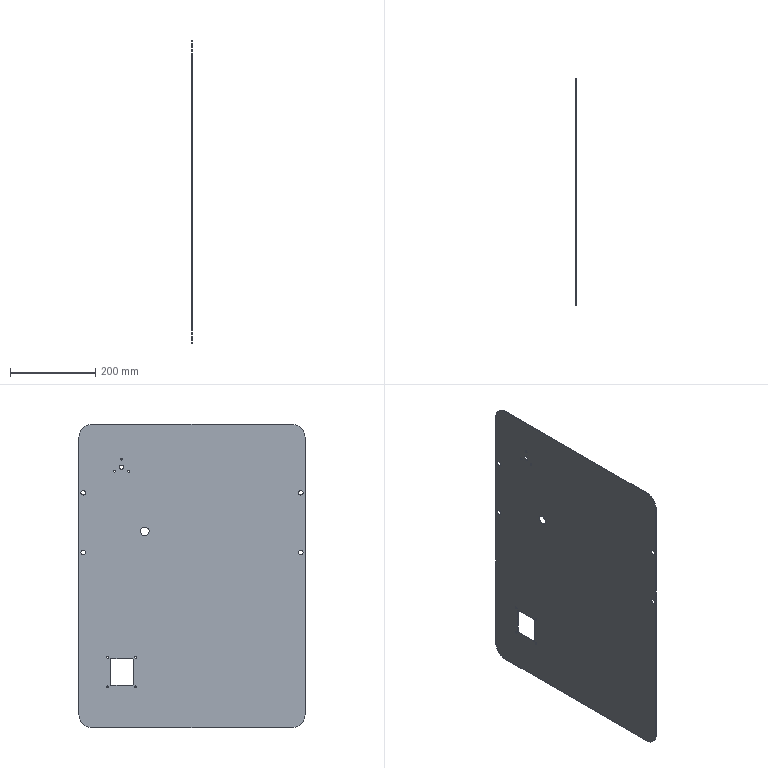Part | STEP file | 冲床-300配套压波_id1022_x_t | 1 solid | 31 faces | box 1.2 x 530 x 710 mm | volume 445518 mm3 | cylinder 21 | plane 10 | commonest cylinder face diameters 4.5 x7 4 x4 10.7 x4 60 x4 10 x1 20 x1
STEP:
#1=CARTESIAN_POINT('',(1921.2,255.,-210.35));
#2=VERTEX_POINT('',#1);
#3=CARTESIAN_POINT('',(1921.2,255.,-205.));
#4=DIRECTION('',(-1.,0.,0.));
#5=DIRECTION('',(0.,0.,-1.));
#6=AXIS2_PLACEMENT_3D('',#3,#4,#5);
#7=CIRCLE('',#6,5.35);
#8=EDGE_CURVE('',#2,#2,#7,.T.);
#9=ORIENTED_EDGE('',*,*,#8,.T.);
#10=EDGE_LOOP('',(#9));
#11=FACE_BOUND('',#10,.T.);
#12=CARTESIAN_POINT('',(1921.2,-255.,-210.35));
#13=VERTEX_POINT('',#12);
#14=CARTESIAN_POINT('',(1921.2,-255.,-205.));
#15=DIRECTION('',(-1.,0.,0.));
#16=DIRECTION('',(0.,0.,-1.));
#17=AXIS2_PLACEMENT_3D('',#14,#15,#16);
#18=CIRCLE('',#17,5.35);
#19=EDGE_CURVE('',#13,#13,#18,.T.);
#20=ORIENTED_EDGE('',*,*,#19,.T.);
#21=EDGE_LOOP('',(#20));
#22=FACE_BOUND('',#21,.T.);
#23=CARTESIAN_POINT('',(1921.2,-255.,-350.35));
#24=VERTEX_POINT('',#23);
#25=CARTESIAN_POINT('',(1921.2,-255.,-345.));
#26=DIRECTION('',(-1.,0.,0.));
#27=DIRECTION('',(0.,0.,-1.));
#28=AXIS2_PLACEMENT_3D('',#25,#26,#27);
#29=CIRCLE('',#28,5.35);
#30=EDGE_CURVE('',#24,#24,#29,.T.);
#31=ORIENTED_EDGE('',*,*,#30,.T.);
#32=EDGE_LOOP('',(#31));
#33=FACE_BOUND('',#32,.T.);
#34=CARTESIAN_POINT('',(1921.2,255.,-350.35));
#35=VERTEX_POINT('',#34);
#36=CARTESIAN_POINT('',(1921.2,255.,-345.));
#37=DIRECTION('',(-1.,0.,0.));
#38=DIRECTION('',(0.,0.,-1.));
#39=AXIS2_PLACEMENT_3D('',#36,#37,#38);
#40=CIRCLE('',#39,5.35);
#41=EDGE_CURVE('',#35,#35,#40,.T.);
#42=ORIENTED_EDGE('',*,*,#41,.T.);
#43=EDGE_LOOP('',(#42));
#44=FACE_BOUND('',#43,.T.);
#45=CARTESIAN_POINT('',(1921.2,181.454,-152.25));
#46=VERTEX_POINT('',#45);
#47=CARTESIAN_POINT('',(1921.2,181.454,-154.5));
#48=DIRECTION('',(1.,0.,0.));
#49=DIRECTION('',(0.,0.,1.));
#50=AXIS2_PLACEMENT_3D('',#47,#48,#49);
#51=CIRCLE('',#50,2.25);
#52=EDGE_CURVE('',#46,#46,#51,.T.);
#53=ORIENTED_EDGE('',*,*,#52,.F.);
#54=EDGE_LOOP('',(#53));
#55=FACE_BOUND('',#54,.T.);
#56=CARTESIAN_POINT('',(1921.2,165.,-123.75));
#57=VERTEX_POINT('',#56);
#58=CARTESIAN_POINT('',(1921.2,165.,-126.));
#59=DIRECTION('',(1.,0.,0.));
#60=DIRECTION('',(0.,0.,1.));
#61=AXIS2_PLACEMENT_3D('',#58,#59,#60);
#62=CIRCLE('',#61,2.25);
#63=EDGE_CURVE('',#57,#57,#62,.T.);
#64=ORIENTED_EDGE('',*,*,#63,.F.);
#65=EDGE_LOOP('',(#64));
#66=FACE_BOUND('',#65,.T.);
#67=CARTESIAN_POINT('',(1921.2,165.,-140.));
#68=VERTEX_POINT('',#67);
#69=CARTESIAN_POINT('',(1921.2,165.,-145.));
#70=DIRECTION('',(1.,0.,0.));
#71=DIRECTION('',(0.,0.,1.));
#72=AXIS2_PLACEMENT_3D('',#69,#70,#71);
#73=CIRCLE('',#72,5.);
#74=EDGE_CURVE('',#68,#68,#73,.T.);
#75=ORIENTED_EDGE('',*,*,#74,.F.);
#76=EDGE_LOOP('',(#75));
#77=FACE_BOUND('',#76,.T.);
#78=CARTESIAN_POINT('',(1921.2,148.546,-152.25));
#79=VERTEX_POINT('',#78);
#80=CARTESIAN_POINT('',(1921.2,148.546,-154.5));
#81=DIRECTION('',(1.,0.,0.));
#82=DIRECTION('',(0.,0.,1.));
#83=AXIS2_PLACEMENT_3D('',#80,#81,#82);
#84=CIRCLE('',#83,2.25);
#85=EDGE_CURVE('',#79,#79,#84,.T.);
#86=ORIENTED_EDGE('',*,*,#85,.F.);
#87=EDGE_LOOP('',(#86));
#88=FACE_BOUND('',#87,.T.);
#89=CARTESIAN_POINT('',(1921.2,110.599,-305.243));
#90=VERTEX_POINT('',#89);
#91=CARTESIAN_POINT('',(1921.2,110.599,-295.243));
#92=DIRECTION('',(-1.,0.,0.));
#93=DIRECTION('',(0.,0.,-1.));
#94=AXIS2_PLACEMENT_3D('',#91,#92,#93);
#95=CIRCLE('',#94,10.);
#96=EDGE_CURVE('',#90,#90,#95,.T.);
#97=ORIENTED_EDGE('',*,*,#96,.T.);
#98=EDGE_LOOP('',(#97));
#99=FACE_BOUND('',#98,.T.);
#100=CARTESIAN_POINT('',(1921.2,265.,-725.));
#101=VERTEX_POINT('',#100);
#102=CARTESIAN_POINT('',(1921.2,265.,-75.));
#103=VERTEX_POINT('',#102);
#104=CARTESIAN_POINT('',(1921.2,265.,-45.));
#105=DIRECTION('',(0.,0.,1.));
#106=VECTOR('',#105,1.);
#107=LINE('',#104,#106);
#108=EDGE_CURVE('',#101,#103,#107,.T.);
#109=ORIENTED_EDGE('',*,*,#108,.T.);
#110=CARTESIAN_POINT('',(1921.2,235.,-45.));
#111=VERTEX_POINT('',#110);
#112=CARTESIAN_POINT('',(1921.2,235.,-75.));
#113=DIRECTION('',(1.,0.,0.));
#114=DIRECTION('',(0.,0.,-1.));
#115=AXIS2_PLACEMENT_3D('',#112,#113,#114);
#116=CIRCLE('',#115,30.);
#117=EDGE_CURVE('',#103,#111,#116,.T.);
#118=ORIENTED_EDGE('',*,*,#117,.T.);
#119=CARTESIAN_POINT('',(1921.2,-235.,-45.));
#120=VERTEX_POINT('',#119);
#121=CARTESIAN_POINT('',(1921.2,-255.,-45.));
#122=DIRECTION('',(0.,-1.,0.));
#123=VECTOR('',#122,1.);
#124=LINE('',#121,#123);
#125=EDGE_CURVE('',#111,#120,#124,.T.);
#126=ORIENTED_EDGE('',*,*,#125,.T.);
#127=CARTESIAN_POINT('',(1921.2,-265.,-75.));
#128=VERTEX_POINT('',#127);
#129=CARTESIAN_POINT('',(1921.2,-235.,-75.));
#130=DIRECTION('',(1.,0.,0.));
#131=DIRECTION('',(0.,0.,-1.));
#132=AXIS2_PLACEMENT_3D('',#129,#130,#131);
#133=CIRCLE('',#132,30.);
#134=EDGE_CURVE('',#120,#128,#133,.T.);
#135=ORIENTED_EDGE('',*,*,#134,.T.);
#136=CARTESIAN_POINT('',(1921.2,-265.,-725.));
#137=VERTEX_POINT('',#136);
#138=CARTESIAN_POINT('',(1921.2,-265.,-755.));
#139=DIRECTION('',(0.,0.,-1.));
#140=VECTOR('',#139,1.);
#141=LINE('',#138,#140);
#142=EDGE_CURVE('',#128,#137,#141,.T.);
#143=ORIENTED_EDGE('',*,*,#142,.T.);
#144=CARTESIAN_POINT('',(1921.2,-235.,-755.));
#145=VERTEX_POINT('',#144);
#146=CARTESIAN_POINT('',(1921.2,-235.,-725.));
#147=DIRECTION('',(1.,0.,0.));
#148=DIRECTION('',(0.,0.,-1.));
#149=AXIS2_PLACEMENT_3D('',#146,#147,#148);
#150=CIRCLE('',#149,30.);
#151=EDGE_CURVE('',#137,#145,#150,.T.);
#152=ORIENTED_EDGE('',*,*,#151,.T.);
#153=CARTESIAN_POINT('',(1921.2,235.,-755.));
#154=VERTEX_POINT('',#153);
#155=CARTESIAN_POINT('',(1921.2,255.,-755.));
#156=DIRECTION('',(0.,1.,0.));
#157=VECTOR('',#156,1.);
#158=LINE('',#155,#157);
#159=EDGE_CURVE('',#145,#154,#158,.T.);
#160=ORIENTED_EDGE('',*,*,#159,.T.);
#161=CARTESIAN_POINT('',(1921.2,235.,-725.));
#162=DIRECTION('',(1.,0.,0.));
#163=DIRECTION('',(0.,0.,-1.));
#164=AXIS2_PLACEMENT_3D('',#161,#162,#163);
#165=CIRCLE('',#164,30.);
#166=EDGE_CURVE('',#154,#101,#165,.T.);
#167=ORIENTED_EDGE('',*,*,#166,.T.);
#168=EDGE_LOOP('',(#109,#118,#126,#135,#143,#152,#160,#167));
#169=FACE_BOUND('',#168,.T.);
#170=CARTESIAN_POINT('',(1921.2,192.,-654.5));
#171=VERTEX_POINT('',#170);
#172=CARTESIAN_POINT('',(1921.2,192.,-595.5));
#173=VERTEX_POINT('',#172);
#174=CARTESIAN_POINT('',(1921.2,192.,10.));
#175=DIRECTION('',(0.,0.,1.));
#176=VECTOR('',#175,1.);
#177=LINE('',#174,#176);
#178=EDGE_CURVE('',#171,#173,#177,.T.);
#179=ORIENTED_EDGE('',*,*,#178,.F.);
#180=CARTESIAN_POINT('',(1921.2,190.,-656.5));
#181=VERTEX_POINT('',#180);
#182=CARTESIAN_POINT('',(1921.2,190.,-654.5));
#183=DIRECTION('',(-1.,0.,0.));
#184=DIRECTION('',(0.,0.,-1.));
#185=AXIS2_PLACEMENT_3D('',#182,#183,#184);
#186=CIRCLE('',#185,2.);
#187=EDGE_CURVE('',#171,#181,#186,.T.);
#188=ORIENTED_EDGE('',*,*,#187,.T.);
#189=CARTESIAN_POINT('',(1921.2,140.,-656.5));
#190=VERTEX_POINT('',#189);
#191=CARTESIAN_POINT('',(1921.2,0.,-656.5));
#192=DIRECTION('',(0.,1.,0.));
#193=VECTOR('',#192,1.);
#194=LINE('',#191,#193);
#195=EDGE_CURVE('',#190,#181,#194,.T.);
#196=ORIENTED_EDGE('',*,*,#195,.F.);
#197=CARTESIAN_POINT('',(1921.2,138.,-654.5));
#198=VERTEX_POINT('',#197);
#199=CARTESIAN_POINT('',(1921.2,140.,-654.5));
#200=DIRECTION('',(-1.,0.,0.));
#201=DIRECTION('',(0.,0.,-1.));
#202=AXIS2_PLACEMENT_3D('',#199,#200,#201);
#203=CIRCLE('',#202,2.);
#204=EDGE_CURVE('',#190,#198,#203,.T.);
#205=ORIENTED_EDGE('',*,*,#204,.T.);
#206=CARTESIAN_POINT('',(1921.2,138.,-595.5));
#207=VERTEX_POINT('',#206);
#208=CARTESIAN_POINT('',(1921.2,138.,10.));
#209=DIRECTION('',(0.,0.,-1.));
#210=VECTOR('',#209,1.);
#211=LINE('',#208,#210);
#212=EDGE_CURVE('',#207,#198,#211,.T.);
#213=ORIENTED_EDGE('',*,*,#212,.F.);
#214=CARTESIAN_POINT('',(1921.2,140.,-593.5));
#215=VERTEX_POINT('',#214);
#216=CARTESIAN_POINT('',(1921.2,140.,-595.5));
#217=DIRECTION('',(-1.,0.,0.));
#218=DIRECTION('',(0.,0.,-1.));
#219=AXIS2_PLACEMENT_3D('',#216,#217,#218);
#220=CIRCLE('',#219,2.);
#221=EDGE_CURVE('',#207,#215,#220,.T.);
#222=ORIENTED_EDGE('',*,*,#221,.T.);
#223=CARTESIAN_POINT('',(1921.2,190.,-593.5));
#224=VERTEX_POINT('',#223);
#225=CARTESIAN_POINT('',(1921.2,0.,-593.5));
#226=DIRECTION('',(0.,-1.,0.));
#227=VECTOR('',#226,1.);
#228=LINE('',#225,#227);
#229=EDGE_CURVE('',#224,#215,#228,.T.);
#230=ORIENTED_EDGE('',*,*,#229,.F.);
#231=CARTESIAN_POINT('',(1921.2,190.,-595.5));
#232=DIRECTION('',(-1.,0.,0.));
#233=DIRECTION('',(0.,0.,-1.));
#234=AXIS2_PLACEMENT_3D('',#231,#232,#233);
#235=CIRCLE('',#234,2.);
#236=EDGE_CURVE('',#224,#173,#235,.T.);
#237=ORIENTED_EDGE('',*,*,#236,.T.);
#238=EDGE_LOOP('',(#179,#188,#196,#205,#213,#222,#230,#237));
#239=FACE_BOUND('',#238,.T.);
#240=CARTESIAN_POINT('',(1921.2,132.15,-662.));
#241=VERTEX_POINT('',#240);
#242=CARTESIAN_POINT('',(1921.2,132.15,-659.75));
#243=DIRECTION('',(-1.,0.,0.));
#244=DIRECTION('',(0.,0.,-1.));
#245=AXIS2_PLACEMENT_3D('',#242,#243,#244);
#246=CIRCLE('',#245,2.25);
#247=EDGE_CURVE('',#241,#241,#246,.T.);
#248=ORIENTED_EDGE('',*,*,#247,.T.);
#249=EDGE_LOOP('',(#248));
#250=FACE_BOUND('',#249,.T.);
#251=CARTESIAN_POINT('',(1921.2,197.85,-592.5));
#252=VERTEX_POINT('',#251);
#253=CARTESIAN_POINT('',(1921.2,197.85,-590.25));
#254=DIRECTION('',(1.,0.,0.));
#255=DIRECTION('',(0.,0.,-1.));
#256=AXIS2_PLACEMENT_3D('',#253,#254,#255);
#257=CIRCLE('',#256,2.25);
#258=EDGE_CURVE('',#252,#252,#257,.T.);
#259=ORIENTED_EDGE('',*,*,#258,.F.);
#260=EDGE_LOOP('',(#259));
#261=FACE_BOUND('',#260,.T.);
#262=CARTESIAN_POINT('',(1921.2,132.15,-592.5));
#263=VERTEX_POINT('',#262);
#264=CARTESIAN_POINT('',(1921.2,132.15,-590.25));
#265=DIRECTION('',(1.,0.,0.));
#266=DIRECTION('',(0.,0.,-1.));
#267=AXIS2_PLACEMENT_3D('',#264,#265,#266);
#268=CIRCLE('',#267,2.25);
#269=EDGE_CURVE('',#263,#263,#268,.T.);
#270=ORIENTED_EDGE('',*,*,#269,.F.);
#271=EDGE_LOOP('',(#270));
#272=FACE_BOUND('',#271,.T.);
#273=CARTESIAN_POINT('',(1921.2,197.85,-662.));
#274=VERTEX_POINT('',#273);
#275=CARTESIAN_POINT('',(1921.2,197.85,-659.75));
#276=DIRECTION('',(1.,0.,0.));
#277=DIRECTION('',(0.,0.,-1.));
#278=AXIS2_PLACEMENT_3D('',#275,#276,#277);
#279=CIRCLE('',#278,2.25);
#280=EDGE_CURVE('',#274,#274,#279,.T.);
#281=ORIENTED_EDGE('',*,*,#280,.F.);
#282=EDGE_LOOP('',(#281));
#283=FACE_BOUND('',#282,.T.);
#284=CARTESIAN_POINT('',(1921.2,0.,10.));
#285=DIRECTION('',(1.,0.,0.));
#286=DIRECTION('',(0.,0.,1.));
#287=AXIS2_PLACEMENT_3D('',#284,#285,#286);
#288=PLANE('',#287);
#289=ADVANCED_FACE('',(#11,#22,#33,#44,#55,#66,#77,#88,#99,#169,#239,#250,#261,#272,#283),#288,.T.);
#290=CARTESIAN_POINT('',(1920.,255.,-210.35));
#291=VERTEX_POINT('',#290);
#292=CARTESIAN_POINT('',(1920.,255.,-205.));
#293=DIRECTION('',(-1.,0.,0.));
#294=DIRECTION('',(0.,0.,-1.));
#295=AXIS2_PLACEMENT_3D('',#292,#293,#294);
#296=CIRCLE('',#295,5.35);
#297=EDGE_CURVE('',#291,#291,#296,.T.);
#298=ORIENTED_EDGE('',*,*,#297,.F.);
#299=EDGE_LOOP('',(#298));
#300=FACE_BOUND('',#299,.T.);
#301=CARTESIAN_POINT('',(1920.,-255.,-210.35));
#302=VERTEX_POINT('',#301);
#303=CARTESIAN_POINT('',(1920.,-255.,-205.));
#304=DIRECTION('',(-1.,0.,0.));
#305=DIRECTION('',(0.,0.,-1.));
#306=AXIS2_PLACEMENT_3D('',#303,#304,#305);
#307=CIRCLE('',#306,5.35);
#308=EDGE_CURVE('',#302,#302,#307,.T.);
#309=ORIENTED_EDGE('',*,*,#308,.F.);
#310=EDGE_LOOP('',(#309));
#311=FACE_BOUND('',#310,.T.);
#312=CARTESIAN_POINT('',(1920.,-255.,-350.35));
#313=VERTEX_POINT('',#312);
#314=CARTESIAN_POINT('',(1920.,-255.,-345.));
#315=DIRECTION('',(-1.,0.,0.));
#316=DIRECTION('',(0.,0.,-1.));
#317=AXIS2_PLACEMENT_3D('',#314,#315,#316);
#318=CIRCLE('',#317,5.35);
#319=EDGE_CURVE('',#313,#313,#318,.T.);
#320=ORIENTED_EDGE('',*,*,#319,.F.);
#321=EDGE_LOOP('',(#320));
#322=FACE_BOUND('',#321,.T.);
#323=CARTESIAN_POINT('',(1920.,255.,-350.35));
#324=VERTEX_POINT('',#323);
#325=CARTESIAN_POINT('',(1920.,255.,-345.));
#326=DIRECTION('',(-1.,0.,0.));
#327=DIRECTION('',(0.,0.,-1.));
#328=AXIS2_PLACEMENT_3D('',#325,#326,#327);
#329=CIRCLE('',#328,5.35);
#330=EDGE_CURVE('',#324,#324,#329,.T.);
#331=ORIENTED_EDGE('',*,*,#330,.F.);
#332=EDGE_LOOP('',(#331));
#333=FACE_BOUND('',#332,.T.);
#334=CARTESIAN_POINT('',(1920.,138.,-595.5));
#335=VERTEX_POINT('',#334);
#336=CARTESIAN_POINT('',(1920.,138.,-654.5));
#337=VERTEX_POINT('',#336);
#338=CARTESIAN_POINT('',(1920.,138.,10.));
#339=DIRECTION('',(0.,0.,-1.));
#340=VECTOR('',#339,1.);
#341=LINE('',#338,#340);
#342=EDGE_CURVE('',#335,#337,#341,.T.);
#343=ORIENTED_EDGE('',*,*,#342,.T.);
#344=CARTESIAN_POINT('',(1920.,140.,-656.5));
#345=VERTEX_POINT('',#344);
#346=CARTESIAN_POINT('',(1920.,140.,-654.5));
#347=DIRECTION('',(1.,0.,0.));
#348=DIRECTION('',(0.,0.,-1.));
#349=AXIS2_PLACEMENT_3D('',#346,#347,#348);
#350=CIRCLE('',#349,2.);
#351=EDGE_CURVE('',#337,#345,#350,.T.);
#352=ORIENTED_EDGE('',*,*,#351,.T.);
#353=CARTESIAN_POINT('',(1920.,190.,-656.5));
#354=VERTEX_POINT('',#353);
#355=CARTESIAN_POINT('',(1920.,0.,-656.5));
#356=DIRECTION('',(0.,1.,0.));
#357=VECTOR('',#356,1.);
#358=LINE('',#355,#357);
#359=EDGE_CURVE('',#345,#354,#358,.T.);
#360=ORIENTED_EDGE('',*,*,#359,.T.);
#361=CARTESIAN_POINT('',(1920.,192.,-654.5));
#362=VERTEX_POINT('',#361);
#363=CARTESIAN_POINT('',(1920.,190.,-654.5));
#364=DIRECTION('',(1.,0.,0.));
#365=DIRECTION('',(0.,0.,-1.));
#366=AXIS2_PLACEMENT_3D('',#363,#364,#365);
#367=CIRCLE('',#366,2.);
#368=EDGE_CURVE('',#354,#362,#367,.T.);
#369=ORIENTED_EDGE('',*,*,#368,.T.);
#370=CARTESIAN_POINT('',(1920.,192.,-595.5));
#371=VERTEX_POINT('',#370);
#372=CARTESIAN_POINT('',(1920.,192.,10.));
#373=DIRECTION('',(0.,0.,1.));
#374=VECTOR('',#373,1.);
#375=LINE('',#372,#374);
#376=EDGE_CURVE('',#362,#371,#375,.T.);
#377=ORIENTED_EDGE('',*,*,#376,.T.);
#378=CARTESIAN_POINT('',(1920.,190.,-593.5));
#379=VERTEX_POINT('',#378);
#380=CARTESIAN_POINT('',(1920.,190.,-595.5));
#381=DIRECTION('',(1.,0.,0.));
#382=DIRECTION('',(0.,0.,-1.));
#383=AXIS2_PLACEMENT_3D('',#380,#381,#382);
#384=CIRCLE('',#383,2.);
#385=EDGE_CURVE('',#371,#379,#384,.T.);
#386=ORIENTED_EDGE('',*,*,#385,.T.);
#387=CARTESIAN_POINT('',(1920.,140.,-593.5));
#388=VERTEX_POINT('',#387);
#389=CARTESIAN_POINT('',(1920.,0.,-593.5));
#390=DIRECTION('',(0.,-1.,0.));
#391=VECTOR('',#390,1.);
#392=LINE('',#389,#391);
#393=EDGE_CURVE('',#379,#388,#392,.T.);
#394=ORIENTED_EDGE('',*,*,#393,.T.);
#395=CARTESIAN_POINT('',(1920.,140.,-595.5));
#396=DIRECTION('',(1.,0.,0.));
#397=DIRECTION('',(0.,0.,-1.));
#398=AXIS2_PLACEMENT_3D('',#395,#396,#397);
#399=CIRCLE('',#398,2.);
#400=EDGE_CURVE('',#388,#335,#399,.T.);
#401=ORIENTED_EDGE('',*,*,#400,.T.);
#402=EDGE_LOOP('',(#343,#352,#360,#369,#377,#386,#394,#401));
#403=FACE_BOUND('',#402,.T.);
#404=CARTESIAN_POINT('',(1920.,197.85,-662.));
#405=VERTEX_POINT('',#404);
#406=CARTESIAN_POINT('',(1920.,197.85,-659.75));
#407=DIRECTION('',(1.,0.,0.));
#408=DIRECTION('',(0.,0.,-1.));
#409=AXIS2_PLACEMENT_3D('',#406,#407,#408);
#410=CIRCLE('',#409,2.25);
#411=EDGE_CURVE('',#405,#405,#410,.T.);
#412=ORIENTED_EDGE('',*,*,#411,.T.);
#413=EDGE_LOOP('',(#412));
#414=FACE_BOUND('',#413,.T.);
#415=CARTESIAN_POINT('',(1920.,132.15,-592.5));
#416=VERTEX_POINT('',#415);
#417=CARTESIAN_POINT('',(1920.,132.15,-590.25));
#418=DIRECTION('',(1.,0.,0.));
#419=DIRECTION('',(0.,0.,-1.));
#420=AXIS2_PLACEMENT_3D('',#417,#418,#419);
#421=CIRCLE('',#420,2.25);
#422=EDGE_CURVE('',#416,#416,#421,.T.);
#423=ORIENTED_EDGE('',*,*,#422,.T.);
#424=EDGE_LOOP('',(#423));
#425=FACE_BOUND('',#424,.T.);
#426=CARTESIAN_POINT('',(1920.,197.85,-592.5));
#427=VERTEX_POINT('',#426);
#428=CARTESIAN_POINT('',(1920.,197.85,-590.25));
#429=DIRECTION('',(1.,0.,0.));
#430=DIRECTION('',(0.,0.,-1.));
#431=AXIS2_PLACEMENT_3D('',#428,#429,#430);
#432=CIRCLE('',#431,2.25);
#433=EDGE_CURVE('',#427,#427,#432,.T.);
#434=ORIENTED_EDGE('',*,*,#433,.T.);
#435=EDGE_LOOP('',(#434));
#436=FACE_BOUND('',#435,.T.);
#437=CARTESIAN_POINT('',(1920.,235.,-45.));
#438=VERTEX_POINT('',#437);
#439=CARTESIAN_POINT('',(1920.,265.,-75.));
#440=VERTEX_POINT('',#439);
#441=CARTESIAN_POINT('',(1920.,235.,-75.));
#442=DIRECTION('',(-1.,0.,0.));
#443=DIRECTION('',(0.,0.,-1.));
#444=AXIS2_PLACEMENT_3D('',#441,#442,#443);
#445=CIRCLE('',#444,30.);
#446=EDGE_CURVE('',#438,#440,#445,.T.);
#447=ORIENTED_EDGE('',*,*,#446,.T.);
#448=CARTESIAN_POINT('',(1920.,265.,-725.));
#449=VERTEX_POINT('',#448);
#450=CARTESIAN_POINT('',(1920.,265.,-45.));
#451=DIRECTION('',(0.,0.,1.));
#452=VECTOR('',#451,1.);
#453=LINE('',#450,#452);
#454=EDGE_CURVE('',#449,#440,#453,.T.);
#455=ORIENTED_EDGE('',*,*,#454,.F.);
#456=CARTESIAN_POINT('',(1920.,235.,-755.));
#457=VERTEX_POINT('',#456);
#458=CARTESIAN_POINT('',(1920.,235.,-725.));
#459=DIRECTION('',(-1.,0.,0.));
#460=DIRECTION('',(0.,0.,-1.));
#461=AXIS2_PLACEMENT_3D('',#458,#459,#460);
#462=CIRCLE('',#461,30.);
#463=EDGE_CURVE('',#449,#457,#462,.T.);
#464=ORIENTED_EDGE('',*,*,#463,.T.);
#465=CARTESIAN_POINT('',(1920.,-235.,-755.));
#466=VERTEX_POINT('',#465);
#467=CARTESIAN_POINT('',(1920.,255.,-755.));
#468=DIRECTION('',(0.,1.,0.));
#469=VECTOR('',#468,1.);
#470=LINE('',#467,#469);
#471=EDGE_CURVE('',#466,#457,#470,.T.);
#472=ORIENTED_EDGE('',*,*,#471,.F.);
#473=CARTESIAN_POINT('',(1920.,-265.,-725.));
#474=VERTEX_POINT('',#473);
#475=CARTESIAN_POINT('',(1920.,-235.,-725.));
#476=DIRECTION('',(-1.,0.,0.));
#477=DIRECTION('',(0.,0.,-1.));
#478=AXIS2_PLACEMENT_3D('',#475,#476,#477);
#479=CIRCLE('',#478,30.);
#480=EDGE_CURVE('',#466,#474,#479,.T.);
#481=ORIENTED_EDGE('',*,*,#480,.T.);
#482=CARTESIAN_POINT('',(1920.,-265.,-75.));
#483=VERTEX_POINT('',#482);
#484=CARTESIAN_POINT('',(1920.,-265.,-755.));
#485=DIRECTION('',(0.,0.,-1.));
#486=VECTOR('',#485,1.);
#487=LINE('',#484,#486);
#488=EDGE_CURVE('',#483,#474,#487,.T.);
#489=ORIENTED_EDGE('',*,*,#488,.F.);
#490=CARTESIAN_POINT('',(1920.,-235.,-45.));
#491=VERTEX_POINT('',#490);
#492=CARTESIAN_POINT('',(1920.,-235.,-75.));
#493=DIRECTION('',(-1.,0.,0.));
#494=DIRECTION('',(0.,0.,-1.));
#495=AXIS2_PLACEMENT_3D('',#492,#493,#494);
#496=CIRCLE('',#495,30.);
#497=EDGE_CURVE('',#483,#491,#496,.T.);
#498=ORIENTED_EDGE('',*,*,#497,.T.);
#499=CARTESIAN_POINT('',(1920.,-255.,-45.));
#500=DIRECTION('',(0.,-1.,0.));
#501=VECTOR('',#500,1.);
#502=LINE('',#499,#501);
#503=EDGE_CURVE('',#438,#491,#502,.T.);
#504=ORIENTED_EDGE('',*,*,#503,.F.);
#505=EDGE_LOOP('',(#447,#455,#464,#472,#481,#489,#498,#504));
#506=FACE_BOUND('',#505,.T.);
#507=CARTESIAN_POINT('',(1920.,181.454,-156.75));
#508=VERTEX_POINT('',#507);
#509=CARTESIAN_POINT('',(1920.,181.454,-154.5));
#510=DIRECTION('',(1.,0.,0.));
#511=DIRECTION('',(0.,0.,-1.));
#512=AXIS2_PLACEMENT_3D('',#509,#510,#511);
#513=CIRCLE('',#512,2.25);
#514=EDGE_CURVE('',#508,#508,#513,.T.);
#515=ORIENTED_EDGE('',*,*,#514,.T.);
#516=EDGE_LOOP('',(#515));
#517=FACE_BOUND('',#516,.T.);
#518=CARTESIAN_POINT('',(1920.,165.,-128.25));
#519=VERTEX_POINT('',#518);
#520=CARTESIAN_POINT('',(1920.,165.,-126.));
#521=DIRECTION('',(1.,0.,0.));
#522=DIRECTION('',(0.,0.,-1.));
#523=AXIS2_PLACEMENT_3D('',#520,#521,#522);
#524=CIRCLE('',#523,2.25);
#525=EDGE_CURVE('',#519,#519,#524,.T.);
#526=ORIENTED_EDGE('',*,*,#525,.T.);
#527=EDGE_LOOP('',(#526));
#528=FACE_BOUND('',#527,.T.);
#529=CARTESIAN_POINT('',(1920.,165.,-150.));
#530=VERTEX_POINT('',#529);
#531=CARTESIAN_POINT('',(1920.,165.,-145.));
#532=DIRECTION('',(1.,0.,0.));
#533=DIRECTION('',(0.,0.,-1.));
#534=AXIS2_PLACEMENT_3D('',#531,#532,#533);
#535=CIRCLE('',#534,5.);
#536=EDGE_CURVE('',#530,#530,#535,.T.);
#537=ORIENTED_EDGE('',*,*,#536,.T.);
#538=EDGE_LOOP('',(#537));
#539=FACE_BOUND('',#538,.T.);
#540=CARTESIAN_POINT('',(1920.,148.546,-156.75));
#541=VERTEX_POINT('',#540);
#542=CARTESIAN_POINT('',(1920.,148.546,-154.5));
#543=DIRECTION('',(1.,0.,0.));
#544=DIRECTION('',(0.,0.,-1.));
#545=AXIS2_PLACEMENT_3D('',#542,#543,#544);
#546=CIRCLE('',#545,2.25);
#547=EDGE_CURVE('',#541,#541,#546,.T.);
#548=ORIENTED_EDGE('',*,*,#547,.T.);
#549=EDGE_LOOP('',(#548));
#550=FACE_BOUND('',#549,.T.);
#551=CARTESIAN_POINT('',(1920.,110.599,-305.243));
#552=VERTEX_POINT('',#551);
#553=CARTESIAN_POINT('',(1920.,110.599,-295.243));
#554=DIRECTION('',(1.,0.,0.));
#555=DIRECTION('',(0.,0.,-1.));
#556=AXIS2_PLACEMENT_3D('',#553,#554,#555);
#557=CIRCLE('',#556,10.);
#558=EDGE_CURVE('',#552,#552,#557,.T.);
#559=ORIENTED_EDGE('',*,*,#558,.T.);
#560=EDGE_LOOP('',(#559));
#561=FACE_BOUND('',#560,.T.);
#562=CARTESIAN_POINT('',(1920.,132.15,-662.));
#563=VERTEX_POINT('',#562);
#564=CARTESIAN_POINT('',(1920.,132.15,-659.75));
#565=DIRECTION('',(-1.,0.,0.));
#566=DIRECTION('',(0.,0.,-1.));
#567=AXIS2_PLACEMENT_3D('',#564,#565,#566);
#568=CIRCLE('',#567,2.25);
#569=EDGE_CURVE('',#563,#563,#568,.T.);
#570=ORIENTED_EDGE('',*,*,#569,.F.);
#571=EDGE_LOOP('',(#570));
#572=FACE_BOUND('',#571,.T.);
#573=CARTESIAN_POINT('',(1920.,0.,10.));
#574=DIRECTION('',(1.,0.,0.));
#575=DIRECTION('',(0.,0.,1.));
#576=AXIS2_PLACEMENT_3D('',#573,#574,#575);
#577=PLANE('',#576);
#578=ADVANCED_FACE('',(#300,#311,#322,#333,#403,#414,#425,#436,#506,#517,#528,#539,#550,#561,#572),#577,.F.);
#579=ORIENTED_EDGE('',*,*,#454,.T.);
#580=CARTESIAN_POINT('',(1920.,265.,-75.));
#581=DIRECTION('',(1.,0.,0.));
#582=VECTOR('',#581,1.);
#583=LINE('',#580,#582);
#584=EDGE_CURVE('',#440,#103,#583,.T.);
#585=ORIENTED_EDGE('',*,*,#584,.T.);
#586=ORIENTED_EDGE('',*,*,#108,.F.);
#587=CARTESIAN_POINT('',(1920.,265.,-725.));
#588=DIRECTION('',(-1.,0.,0.));
#589=VECTOR('',#588,1.);
#590=LINE('',#587,#589);
#591=EDGE_CURVE('',#101,#449,#590,.T.);
#592=ORIENTED_EDGE('',*,*,#591,.T.);
#593=EDGE_LOOP('',(#579,#585,#586,#592));
#594=FACE_OUTER_BOUND('',#593,.T.);
#595=CARTESIAN_POINT('',(1920.,265.,-45.));
#596=DIRECTION('',(0.,1.,0.));
#597=DIRECTION('',(0.,0.,1.));
#598=AXIS2_PLACEMENT_3D('',#595,#596,#597);
#599=PLANE('',#598);
#600=ADVANCED_FACE('',(#594),#599,.T.);
#601=CARTESIAN_POINT('',(1920.,-265.,-725.));
#602=DIRECTION('',(1.,0.,0.));
#603=VECTOR('',#602,1.);
#604=LINE('',#601,#603);
#605=EDGE_CURVE('',#474,#137,#604,.T.);
#606=ORIENTED_EDGE('',*,*,#605,.T.);
#607=ORIENTED_EDGE('',*,*,#142,.F.);
#608=CARTESIAN_POINT('',(1920.,-265.,-75.));
#609=DIRECTION('',(-1.,0.,0.));
#610=VECTOR('',#609,1.);
#611=LINE('',#608,#610);
#612=EDGE_CURVE('',#128,#483,#611,.T.);
#613=ORIENTED_EDGE('',*,*,#612,.T.);
#614=ORIENTED_EDGE('',*,*,#488,.T.);
#615=EDGE_LOOP('',(#606,#607,#613,#614));
#616=FACE_OUTER_BOUND('',#615,.T.);
#617=CARTESIAN_POINT('',(1920.,-265.,-755.));
#618=DIRECTION('',(0.,-1.,0.));
#619=DIRECTION('',(0.,0.,-1.));
#620=AXIS2_PLACEMENT_3D('',#617,#618,#619);
#621=PLANE('',#620);
#622=ADVANCED_FACE('',(#616),#621,.T.);
#623=ORIENTED_EDGE('',*,*,#96,.F.);
#624=EDGE_LOOP('',(#623));
#625=FACE_BOUND('',#624,.T.);
#626=ORIENTED_EDGE('',*,*,#558,.F.);
#627=EDGE_LOOP('',(#626));
#628=FACE_BOUND('',#627,.T.);
#629=CARTESIAN_POINT('',(1929.2,110.599,-295.243));
#630=DIRECTION('',(-1.,0.,0.));
#631=DIRECTION('',(0.,0.,1.));
#632=AXIS2_PLACEMENT_3D('',#629,#630,#631);
#633=CYLINDRICAL_SURFACE('',#632,10.);
#634=ADVANCED_FACE('',(#625,#628),#633,.F.);
#635=ORIENTED_EDGE('',*,*,#125,.F.);
#636=CARTESIAN_POINT('',(1920.,235.,-45.));
#637=DIRECTION('',(-1.,0.,0.));
#638=VECTOR('',#637,1.);
#639=LINE('',#636,#638);
#640=EDGE_CURVE('',#111,#438,#639,.T.);
#641=ORIENTED_EDGE('',*,*,#640,.T.);
#642=ORIENTED_EDGE('',*,*,#503,.T.);
#643=CARTESIAN_POINT('',(1920.,-235.,-45.));
#644=DIRECTION('',(1.,0.,0.));
#645=VECTOR('',#644,1.);
#646=LINE('',#643,#645);
#647=EDGE_CURVE('',#491,#120,#646,.T.);
#648=ORIENTED_EDGE('',*,*,#647,.T.);
#649=EDGE_LOOP('',(#635,#641,#642,#648));
#650=FACE_OUTER_BOUND('',#649,.T.);
#651=CARTESIAN_POINT('',(1920.,-255.,-45.));
#652=DIRECTION('',(0.,0.,1.));
#653=DIRECTION('',(-1.,0.,0.));
#654=AXIS2_PLACEMENT_3D('',#651,#652,#653);
#655=PLANE('',#654);
#656=ADVANCED_FACE('',(#650),#655,.T.);
#657=ORIENTED_EDGE('',*,*,#471,.T.);
#658=CARTESIAN_POINT('',(1920.,235.,-755.));
#659=DIRECTION('',(1.,0.,0.));
#660=VECTOR('',#659,1.);
#661=LINE('',#658,#660);
#662=EDGE_CURVE('',#457,#154,#661,.T.);
#663=ORIENTED_EDGE('',*,*,#662,.T.);
#664=ORIENTED_EDGE('',*,*,#159,.F.);
#665=CARTESIAN_POINT('',(1920.,-235.,-755.));
#666=DIRECTION('',(-1.,0.,0.));
#667=VECTOR('',#666,1.);
#668=LINE('',#665,#667);
#669=EDGE_CURVE('',#145,#466,#668,.T.);
#670=ORIENTED_EDGE('',*,*,#669,.T.);
#671=EDGE_LOOP('',(#657,#663,#664,#670));
#672=FACE_OUTER_BOUND('',#671,.T.);
#673=CARTESIAN_POINT('',(1920.,255.,-755.));
#674=DIRECTION('',(0.,0.,-1.));
#675=DIRECTION('',(1.,0.,0.));
#676=AXIS2_PLACEMENT_3D('',#673,#674,#675);
#677=PLANE('',#676);
#678=ADVANCED_FACE('',(#672),#677,.T.);
#679=ORIENTED_EDGE('',*,*,#85,.T.);
#680=EDGE_LOOP('',(#679));
#681=FACE_BOUND('',#680,.T.);
#682=ORIENTED_EDGE('',*,*,#547,.F.);
#683=EDGE_LOOP('',(#682));
#684=FACE_BOUND('',#683,.T.);
#685=CARTESIAN_POINT('',(1887.2,148.546,-154.5));
#686=DIRECTION('',(1.,0.,0.));
#687=DIRECTION('',(0.,0.,1.));
#688=AXIS2_PLACEMENT_3D('',#685,#686,#687);
#689=CYLINDRICAL_SURFACE('',#688,2.25);
#690=ADVANCED_FACE('',(#681,#684),#689,.F.);
#691=ORIENTED_EDGE('',*,*,#74,.T.);
#692=EDGE_LOOP('',(#691));
#693=FACE_BOUND('',#692,.T.);
#694=ORIENTED_EDGE('',*,*,#536,.F.);
#695=EDGE_LOOP('',(#694));
#696=FACE_BOUND('',#695,.T.);
#697=CARTESIAN_POINT('',(1887.2,165.,-145.));
#698=DIRECTION('',(1.,0.,0.));
#699=DIRECTION('',(0.,0.,1.));
#700=AXIS2_PLACEMENT_3D('',#697,#698,#699);
#701=CYLINDRICAL_SURFACE('',#700,5.);
#702=ADVANCED_FACE('',(#693,#696),#701,.F.);
#703=ORIENTED_EDGE('',*,*,#63,.T.);
#704=EDGE_LOOP('',(#703));
#705=FACE_BOUND('',#704,.T.);
#706=ORIENTED_EDGE('',*,*,#525,.F.);
#707=EDGE_LOOP('',(#706));
#708=FACE_BOUND('',#707,.T.);
#709=CARTESIAN_POINT('',(1887.2,165.,-126.));
#710=DIRECTION('',(1.,0.,0.));
#711=DIRECTION('',(0.,0.,1.));
#712=AXIS2_PLACEMENT_3D('',#709,#710,#711);
#713=CYLINDRICAL_SURFACE('',#712,2.25);
#714=ADVANCED_FACE('',(#705,#708),#713,.F.);
#715=ORIENTED_EDGE('',*,*,#52,.T.);
#716=EDGE_LOOP('',(#715));
#717=FACE_BOUND('',#716,.T.);
#718=ORIENTED_EDGE('',*,*,#514,.F.);
#719=EDGE_LOOP('',(#718));
#720=FACE_BOUND('',#719,.T.);
#721=CARTESIAN_POINT('',(1887.2,181.454,-154.5));
#722=DIRECTION('',(1.,0.,0.));
#723=DIRECTION('',(0.,0.,1.));
#724=AXIS2_PLACEMENT_3D('',#721,#722,#723);
#725=CYLINDRICAL_SURFACE('',#724,2.25);
#726=ADVANCED_FACE('',(#717,#720),#725,.F.);
#727=ORIENTED_EDGE('',*,*,#117,.F.);
#728=ORIENTED_EDGE('',*,*,#584,.F.);
#729=ORIENTED_EDGE('',*,*,#446,.F.);
#730=ORIENTED_EDGE('',*,*,#640,.F.);
#731=EDGE_LOOP('',(#727,#728,#729,#730));
#732=FACE_OUTER_BOUND('',#731,.T.);
#733=CARTESIAN_POINT('',(1920.,235.,-75.));
#734=DIRECTION('',(-1.,0.,0.));
#735=DIRECTION('',(0.,0.,1.));
#736=AXIS2_PLACEMENT_3D('',#733,#734,#735);
#737=CYLINDRICAL_SURFACE('',#736,30.);
#738=ADVANCED_FACE('',(#732),#737,.T.);
#739=ORIENTED_EDGE('',*,*,#134,.F.);
#740=ORIENTED_EDGE('',*,*,#647,.F.);
#741=ORIENTED_EDGE('',*,*,#497,.F.);
#742=ORIENTED_EDGE('',*,*,#612,.F.);
#743=EDGE_LOOP('',(#739,#740,#741,#742));
#744=FACE_OUTER_BOUND('',#743,.T.);
#745=CARTESIAN_POINT('',(1920.,-235.,-75.));
#746=DIRECTION('',(-1.,0.,0.));
#747=DIRECTION('',(0.,0.,1.));
#748=AXIS2_PLACEMENT_3D('',#745,#746,#747);
#749=CYLINDRICAL_SURFACE('',#748,30.);
#750=ADVANCED_FACE('',(#744),#749,.T.);
#751=ORIENTED_EDGE('',*,*,#166,.F.);
#752=ORIENTED_EDGE('',*,*,#662,.F.);
#753=ORIENTED_EDGE('',*,*,#463,.F.);
#754=ORIENTED_EDGE('',*,*,#591,.F.);
#755=EDGE_LOOP('',(#751,#752,#753,#754));
#756=FACE_OUTER_BOUND('',#755,.T.);
#757=CARTESIAN_POINT('',(1920.,235.,-725.));
#758=DIRECTION('',(-1.,0.,0.));
#759=DIRECTION('',(0.,0.,1.));
#760=AXIS2_PLACEMENT_3D('',#757,#758,#759);
#761=CYLINDRICAL_SURFACE('',#760,30.);
#762=ADVANCED_FACE('',(#756),#761,.T.);
#763=ORIENTED_EDGE('',*,*,#151,.F.);
#764=ORIENTED_EDGE('',*,*,#605,.F.);
#765=ORIENTED_EDGE('',*,*,#480,.F.);
#766=ORIENTED_EDGE('',*,*,#669,.F.);
#767=EDGE_LOOP('',(#763,#764,#765,#766));
#768=FACE_OUTER_BOUND('',#767,.T.);
#769=CARTESIAN_POINT('',(1920.,-235.,-725.));
#770=DIRECTION('',(-1.,0.,0.));
#771=DIRECTION('',(0.,0.,1.));
#772=AXIS2_PLACEMENT_3D('',#769,#770,#771);
#773=CYLINDRICAL_SURFACE('',#772,30.);
#774=ADVANCED_FACE('',(#768),#773,.T.);
#775=ORIENTED_EDGE('',*,*,#258,.T.);
#776=EDGE_LOOP('',(#775));
#777=FACE_BOUND('',#776,.T.);
#778=ORIENTED_EDGE('',*,*,#433,.F.);
#779=EDGE_LOOP('',(#778));
#780=FACE_BOUND('',#779,.T.);
#781=CARTESIAN_POINT('',(1859.2,197.85,-590.25));
#782=DIRECTION('',(1.,0.,0.));
#783=DIRECTION('',(0.,0.,-1.));
#784=AXIS2_PLACEMENT_3D('',#781,#782,#783);
#785=CYLINDRICAL_SURFACE('',#784,2.25);
#786=ADVANCED_FACE('',(#777,#780),#785,.F.);
#787=ORIENTED_EDGE('',*,*,#247,.F.);
#788=EDGE_LOOP('',(#787));
#789=FACE_BOUND('',#788,.T.);
#790=ORIENTED_EDGE('',*,*,#569,.T.);
#791=EDGE_LOOP('',(#790));
#792=FACE_BOUND('',#791,.T.);
#793=CARTESIAN_POINT('',(1859.2,132.15,-659.75));
#794=DIRECTION('',(1.,0.,0.));
#795=DIRECTION('',(0.,0.,-1.));
#796=AXIS2_PLACEMENT_3D('',#793,#794,#795);
#797=CYLINDRICAL_SURFACE('',#796,2.25);
#798=ADVANCED_FACE('',(#789,#792),#797,.F.);
#799=ORIENTED_EDGE('',*,*,#269,.T.);
#800=EDGE_LOOP('',(#799));
#801=FACE_BOUND('',#800,.T.);
#802=ORIENTED_EDGE('',*,*,#422,.F.);
#803=EDGE_LOOP('',(#802));
#804=FACE_BOUND('',#803,.T.);
#805=CARTESIAN_POINT('',(1859.2,132.15,-590.25));
#806=DIRECTION('',(1.,0.,0.));
#807=DIRECTION('',(0.,0.,-1.));
#808=AXIS2_PLACEMENT_3D('',#805,#806,#807);
#809=CYLINDRICAL_SURFACE('',#808,2.25);
#810=ADVANCED_FACE('',(#801,#804),#809,.F.);
#811=ORIENTED_EDGE('',*,*,#280,.T.);
#812=EDGE_LOOP('',(#811));
#813=FACE_BOUND('',#812,.T.);
#814=ORIENTED_EDGE('',*,*,#411,.F.);
#815=EDGE_LOOP('',(#814));
#816=FACE_BOUND('',#815,.T.);
#817=CARTESIAN_POINT('',(1859.2,197.85,-659.75));
#818=DIRECTION('',(1.,0.,0.));
#819=DIRECTION('',(0.,0.,-1.));
#820=AXIS2_PLACEMENT_3D('',#817,#818,#819);
#821=CYLINDRICAL_SURFACE('',#820,2.25);
#822=ADVANCED_FACE('',(#813,#816),#821,.F.);
#823=ORIENTED_EDGE('',*,*,#376,.F.);
#824=CARTESIAN_POINT('',(1921.2,192.,-654.5));
#825=DIRECTION('',(1.,0.,0.));
#826=VECTOR('',#825,1.);
#827=LINE('',#824,#826);
#828=EDGE_CURVE('',#362,#171,#827,.T.);
#829=ORIENTED_EDGE('',*,*,#828,.T.);
#830=ORIENTED_EDGE('',*,*,#178,.T.);
#831=CARTESIAN_POINT('',(1920.,192.,-595.5));
#832=DIRECTION('',(-1.,0.,0.));
#833=VECTOR('',#832,1.);
#834=LINE('',#831,#833);
#835=EDGE_CURVE('',#173,#371,#834,.T.);
#836=ORIENTED_EDGE('',*,*,#835,.T.);
#837=EDGE_LOOP('',(#823,#829,#830,#836));
#838=FACE_OUTER_BOUND('',#837,.T.);
#839=CARTESIAN_POINT('',(1901.2,192.,-655.));
#840=DIRECTION('',(0.,1.,0.));
#841=DIRECTION('',(0.,0.,1.));
#842=AXIS2_PLACEMENT_3D('',#839,#840,#841);
#843=PLANE('',#842);
#844=ADVANCED_FACE('',(#838),#843,.F.);
#845=ORIENTED_EDGE('',*,*,#393,.F.);
#846=CARTESIAN_POINT('',(1921.2,190.,-593.5));
#847=DIRECTION('',(1.,0.,0.));
#848=VECTOR('',#847,1.);
#849=LINE('',#846,#848);
#850=EDGE_CURVE('',#379,#224,#849,.T.);
#851=ORIENTED_EDGE('',*,*,#850,.T.);
#852=ORIENTED_EDGE('',*,*,#229,.T.);
#853=CARTESIAN_POINT('',(1920.,140.,-593.5));
#854=DIRECTION('',(-1.,0.,0.));
#855=VECTOR('',#854,1.);
#856=LINE('',#853,#855);
#857=EDGE_CURVE('',#215,#388,#856,.T.);
#858=ORIENTED_EDGE('',*,*,#857,.T.);
#859=EDGE_LOOP('',(#845,#851,#852,#858));
#860=FACE_OUTER_BOUND('',#859,.T.);
#861=CARTESIAN_POINT('',(1901.2,191.25,-593.5));
#862=DIRECTION('',(0.,0.,1.));
#863=DIRECTION('',(1.,0.,0.));
#864=AXIS2_PLACEMENT_3D('',#861,#862,#863);
#865=PLANE('',#864);
#866=ADVANCED_FACE('',(#860),#865,.F.);
#867=ORIENTED_EDGE('',*,*,#212,.T.);
#868=CARTESIAN_POINT('',(1920.,138.,-654.5));
#869=DIRECTION('',(-1.,0.,0.));
#870=VECTOR('',#869,1.);
#871=LINE('',#868,#870);
#872=EDGE_CURVE('',#198,#337,#871,.T.);
#873=ORIENTED_EDGE('',*,*,#872,.T.);
#874=ORIENTED_EDGE('',*,*,#342,.F.);
#875=CARTESIAN_POINT('',(1921.2,138.,-595.5));
#876=DIRECTION('',(1.,0.,0.));
#877=VECTOR('',#876,1.);
#878=LINE('',#875,#877);
#879=EDGE_CURVE('',#335,#207,#878,.T.);
#880=ORIENTED_EDGE('',*,*,#879,.T.);
#881=EDGE_LOOP('',(#867,#873,#874,#880));
#882=FACE_OUTER_BOUND('',#881,.T.);
#883=CARTESIAN_POINT('',(1901.2,138.,-595.));
#884=DIRECTION('',(0.,-1.,0.));
#885=DIRECTION('',(0.,0.,-1.));
#886=AXIS2_PLACEMENT_3D('',#883,#884,#885);
#887=PLANE('',#886);
#888=ADVANCED_FACE('',(#882),#887,.F.);
#889=ORIENTED_EDGE('',*,*,#359,.F.);
#890=CARTESIAN_POINT('',(1921.2,140.,-656.5));
#891=DIRECTION('',(1.,0.,0.));
#892=VECTOR('',#891,1.);
#893=LINE('',#890,#892);
#894=EDGE_CURVE('',#345,#190,#893,.T.);
#895=ORIENTED_EDGE('',*,*,#894,.T.);
#896=ORIENTED_EDGE('',*,*,#195,.T.);
#897=CARTESIAN_POINT('',(1920.,190.,-656.5));
#898=DIRECTION('',(-1.,0.,0.));
#899=VECTOR('',#898,1.);
#900=LINE('',#897,#899);
#901=EDGE_CURVE('',#181,#354,#900,.T.);
#902=ORIENTED_EDGE('',*,*,#901,.T.);
#903=EDGE_LOOP('',(#889,#895,#896,#902));
#904=FACE_OUTER_BOUND('',#903,.T.);
#905=CARTESIAN_POINT('',(1901.2,138.75,-656.5));
#906=DIRECTION('',(0.,0.,-1.));
#907=DIRECTION('',(-1.,0.,0.));
#908=AXIS2_PLACEMENT_3D('',#905,#906,#907);
#909=PLANE('',#908);
#910=ADVANCED_FACE('',(#904),#909,.F.);
#911=ORIENTED_EDGE('',*,*,#204,.F.);
#912=ORIENTED_EDGE('',*,*,#894,.F.);
#913=ORIENTED_EDGE('',*,*,#351,.F.);
#914=ORIENTED_EDGE('',*,*,#872,.F.);
#915=EDGE_LOOP('',(#911,#912,#913,#914));
#916=FACE_OUTER_BOUND('',#915,.T.);
#917=CARTESIAN_POINT('',(1901.2,140.,-654.5));
#918=DIRECTION('',(1.,0.,0.));
#919=DIRECTION('',(0.,0.,-1.));
#920=AXIS2_PLACEMENT_3D('',#917,#918,#919);
#921=CYLINDRICAL_SURFACE('',#920,2.);
#922=ADVANCED_FACE('',(#916),#921,.F.);
#923=ORIENTED_EDGE('',*,*,#187,.F.);
#924=ORIENTED_EDGE('',*,*,#828,.F.);
#925=ORIENTED_EDGE('',*,*,#368,.F.);
#926=ORIENTED_EDGE('',*,*,#901,.F.);
#927=EDGE_LOOP('',(#923,#924,#925,#926));
#928=FACE_OUTER_BOUND('',#927,.T.);
#929=CARTESIAN_POINT('',(1901.2,190.,-654.5));
#930=DIRECTION('',(1.,0.,0.));
#931=DIRECTION('',(0.,0.,-1.));
#932=AXIS2_PLACEMENT_3D('',#929,#930,#931);
#933=CYLINDRICAL_SURFACE('',#932,2.);
#934=ADVANCED_FACE('',(#928),#933,.F.);
#935=ORIENTED_EDGE('',*,*,#236,.F.);
#936=ORIENTED_EDGE('',*,*,#850,.F.);
#937=ORIENTED_EDGE('',*,*,#385,.F.);
#938=ORIENTED_EDGE('',*,*,#835,.F.);
#939=EDGE_LOOP('',(#935,#936,#937,#938));
#940=FACE_OUTER_BOUND('',#939,.T.);
#941=CARTESIAN_POINT('',(1901.2,190.,-595.5));
#942=DIRECTION('',(1.,0.,0.));
#943=DIRECTION('',(0.,0.,-1.));
#944=AXIS2_PLACEMENT_3D('',#941,#942,#943);
#945=CYLINDRICAL_SURFACE('',#944,2.);
#946=ADVANCED_FACE('',(#940),#945,.F.);
#947=ORIENTED_EDGE('',*,*,#221,.F.);
#948=ORIENTED_EDGE('',*,*,#879,.F.);
#949=ORIENTED_EDGE('',*,*,#400,.F.);
#950=ORIENTED_EDGE('',*,*,#857,.F.);
#951=EDGE_LOOP('',(#947,#948,#949,#950));
#952=FACE_OUTER_BOUND('',#951,.T.);
#953=CARTESIAN_POINT('',(1901.2,140.,-595.5));
#954=DIRECTION('',(1.,0.,0.));
#955=DIRECTION('',(0.,0.,-1.));
#956=AXIS2_PLACEMENT_3D('',#953,#954,#955);
#957=CYLINDRICAL_SURFACE('',#956,2.);
#958=ADVANCED_FACE('',(#952),#957,.F.);
#959=ORIENTED_EDGE('',*,*,#41,.F.);
#960=EDGE_LOOP('',(#959));
#961=FACE_BOUND('',#960,.T.);
#962=ORIENTED_EDGE('',*,*,#330,.T.);
#963=EDGE_LOOP('',(#962));
#964=FACE_BOUND('',#963,.T.);
#965=CARTESIAN_POINT('',(1895.,255.,-345.));
#966=DIRECTION('',(1.,0.,0.));
#967=DIRECTION('',(0.,0.,-1.));
#968=AXIS2_PLACEMENT_3D('',#965,#966,#967);
#969=CYLINDRICAL_SURFACE('',#968,5.35);
#970=ADVANCED_FACE('',(#961,#964),#969,.F.);
#971=ORIENTED_EDGE('',*,*,#30,.F.);
#972=EDGE_LOOP('',(#971));
#973=FACE_BOUND('',#972,.T.);
#974=ORIENTED_EDGE('',*,*,#319,.T.);
#975=EDGE_LOOP('',(#974));
#976=FACE_BOUND('',#975,.T.);
#977=CARTESIAN_POINT('',(1895.,-255.,-345.));
#978=DIRECTION('',(1.,0.,0.));
#979=DIRECTION('',(0.,0.,-1.));
#980=AXIS2_PLACEMENT_3D('',#977,#978,#979);
#981=CYLINDRICAL_SURFACE('',#980,5.35);
#982=ADVANCED_FACE('',(#973,#976),#981,.F.);
#983=ORIENTED_EDGE('',*,*,#19,.F.);
#984=EDGE_LOOP('',(#983));
#985=FACE_BOUND('',#984,.T.);
#986=ORIENTED_EDGE('',*,*,#308,.T.);
#987=EDGE_LOOP('',(#986));
#988=FACE_BOUND('',#987,.T.);
#989=CARTESIAN_POINT('',(1895.,-255.,-205.));
#990=DIRECTION('',(1.,0.,0.));
#991=DIRECTION('',(0.,0.,-1.));
#992=AXIS2_PLACEMENT_3D('',#989,#990,#991);
#993=CYLINDRICAL_SURFACE('',#992,5.35);
#994=ADVANCED_FACE('',(#985,#988),#993,.F.);
#995=ORIENTED_EDGE('',*,*,#8,.F.);
#996=EDGE_LOOP('',(#995));
#997=FACE_BOUND('',#996,.T.);
#998=ORIENTED_EDGE('',*,*,#297,.T.);
#999=EDGE_LOOP('',(#998));
#1000=FACE_BOUND('',#999,.T.);
#1001=CARTESIAN_POINT('',(1895.,255.,-205.));
#1002=DIRECTION('',(1.,0.,0.));
#1003=DIRECTION('',(0.,0.,-1.));
#1004=AXIS2_PLACEMENT_3D('',#1001,#1002,#1003);
#1005=CYLINDRICAL_SURFACE('',#1004,5.35);
#1006=ADVANCED_FACE('',(#997,#1000),#1005,.F.);
#1007=CLOSED_SHELL('',(#289,#578,#600,#622,#634,#656,#678,#690,#702,#714,#726,#738,#750,#762,#774,#786,#798,#810,#822,#844,#866,#888,#910,#922,#934,#946,#958,#970,#982,#994,#1006));
#1008=MANIFOLD_SOLID_BREP('',#1007);
#1009=(LENGTH_UNIT()NAMED_UNIT(*)SI_UNIT(.MILLI.,.METRE.));
#1010=UNCERTAINTY_MEASURE_WITH_UNIT(LENGTH_MEASURE(0.00002),#1009,'','');
#1011=(NAMED_UNIT(*)PLANE_ANGLE_UNIT()SI_UNIT($,.RADIAN.));
#1012=PLANE_ANGLE_MEASURE_WITH_UNIT(PLANE_ANGLE_MEASURE(0.01745),#1011);
#1013=DIMENSIONAL_EXPONENTS(0.,0.,0.,0.,0.,0.,0.);
#1014=(CONVERSION_BASED_UNIT('DEGREE',#1012)NAMED_UNIT(#1013)PLANE_ANGLE_UNIT());
#1015=(NAMED_UNIT(*)SI_UNIT($,.STERADIAN.)SOLID_ANGLE_UNIT());
#1016=(GEOMETRIC_REPRESENTATION_CONTEXT(3)GLOBAL_UNCERTAINTY_ASSIGNED_CONTEXT((#1010))GLOBAL_UNIT_ASSIGNED_CONTEXT((#1009,#1014,#1015))REPRESENTATION_CONTEXT('',''));
#1017=ADVANCED_BREP_SHAPE_REPRESENTATION('',(#1008),#1016);